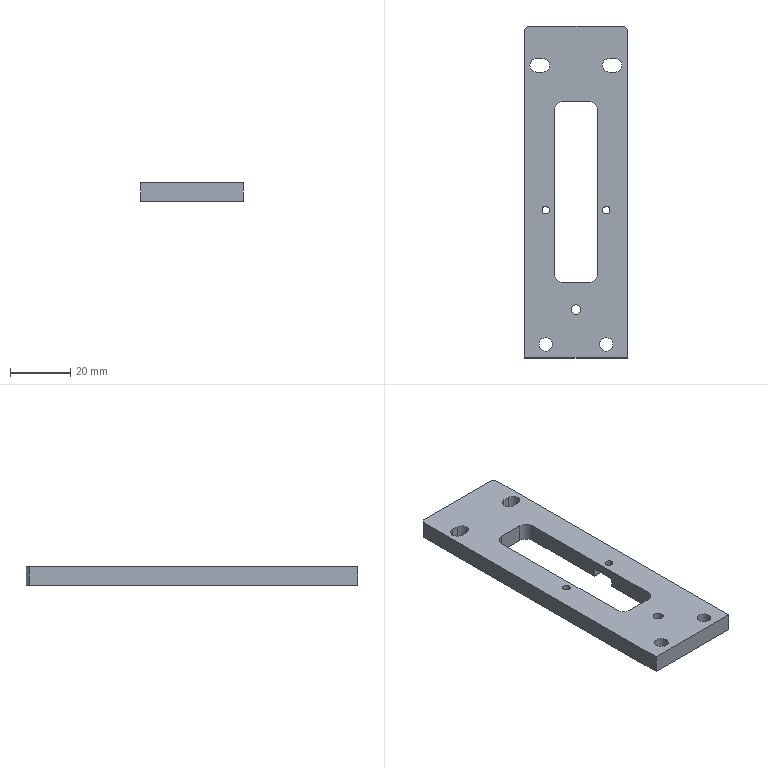Part | SolidWorks | features HoleWzd 3, ICE 3, Chamfer 1, Cut 1, Extrusion 1, Fillet 1 | 1 solid | 50 faces | box 34 x 110 x 6 mm | volume 16362 mm3 | cylinder 26 | plane 24 | commonest cylinder face diameters 4.5 x10 2 x6 2.5 x4 6 x4 3.3 x2